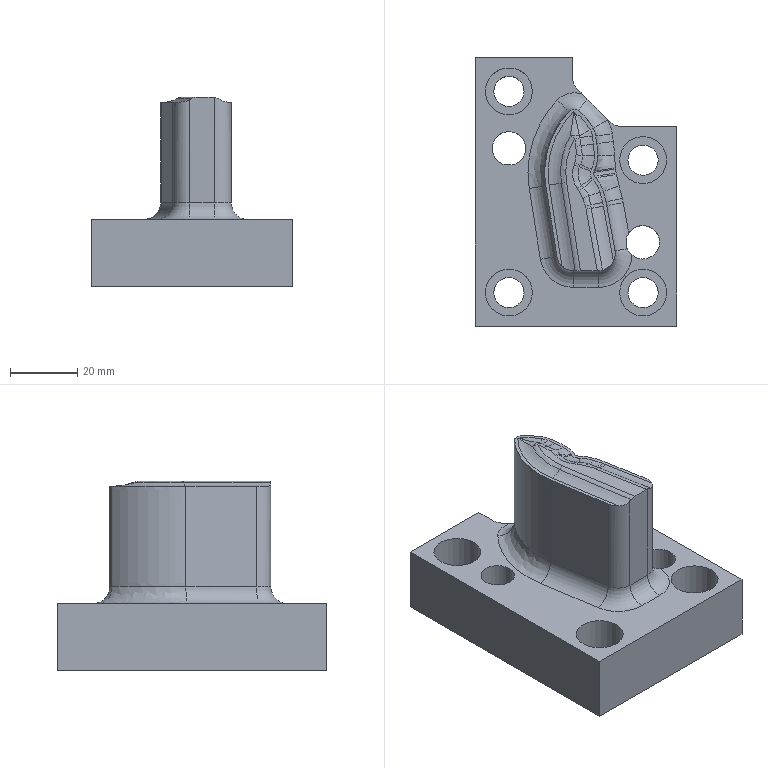Part | STEP file | 1 solid | 92 faces | box 60 x 80 x 56.5 mm | volume 99207 mm3 | cylinder 34 | spline 27 | plane 17 | torus 11 | other 2 | sphere 1 | commonest cylinder face diameters 10 x8 14 x7 9 x4 6 x2 2.518 x1 4 x1